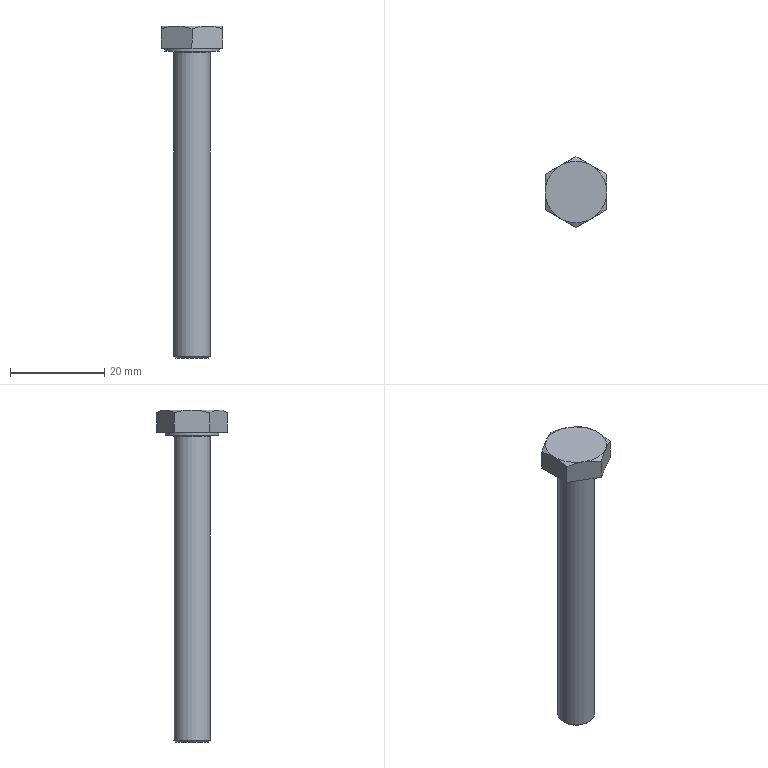Part | NX | features SKETCH 4, EXTRUDE 3, META 3, DATUM_CSYS 2, BLEND 1, CHAMFER 1, LINE 1, SWP104 1, SYMBOLIC_THREAD 1, THREADS 1 | 1 solid | 20 faces | box 13 x 15.011 x 70.3 mm | volume 3821 mm3 | plane 10 | cone 7 | cylinder 2 | torus 1 | commonest cylinder face diameters 7.76 x1 11.47 x1
STEP:
#1=CARTESIAN_POINT('',(4.28,0.,0.));
#2=VERTEX_POINT('',#1);
#3=CARTESIAN_POINT('',(0.,0.,0.));
#4=DIRECTION('',(0.,0.,1.));
#5=DIRECTION('',(1.,0.,0.));
#6=AXIS2_PLACEMENT_3D('',#3,#4,#5);
#7=CIRCLE('',#6,4.28);
#8=EDGE_CURVE('',#2,#2,#7,.T.);
#9=ORIENTED_EDGE('',*,*,#8,.T.);
#10=EDGE_LOOP('',(#9));
#11=FACE_BOUND('',#10,.T.);
#12=CARTESIAN_POINT('',(5.735,0.,0.));
#13=VERTEX_POINT('',#12);
#14=CARTESIAN_POINT('',(0.,0.,0.));
#15=DIRECTION('',(0.,0.,1.));
#16=DIRECTION('',(1.,0.,0.));
#17=AXIS2_PLACEMENT_3D('',#14,#15,#16);
#18=CIRCLE('',#17,5.735);
#19=EDGE_CURVE('',#13,#13,#18,.T.);
#20=ORIENTED_EDGE('',*,*,#19,.F.);
#21=EDGE_LOOP('',(#20));
#22=FACE_BOUND('',#21,.T.);
#23=CARTESIAN_POINT('',(0.,0.,0.));
#24=DIRECTION('',(0.,0.,1.));
#25=DIRECTION('',(1.,0.,0.));
#26=AXIS2_PLACEMENT_3D('',#23,#24,#25);
#27=PLANE('',#26);
#28=ADVANCED_FACE('',(#11,#22),#27,.F.);
#29=CARTESIAN_POINT('',(6.5,3.753,4.719));
#30=VERTEX_POINT('',#29);
#31=CARTESIAN_POINT('',(3.25,5.629,5.3));
#32=VERTEX_POINT('',#31);
#33=CARTESIAN_POINT('',(6.5,3.753,4.719));
#34=CARTESIAN_POINT('',(5.437,4.367,5.074));
#35=CARTESIAN_POINT('',(4.357,4.99,5.3));
#36=CARTESIAN_POINT('',(3.25,5.629,5.3));
#37=B_SPLINE_CURVE_WITH_KNOTS('',3,(#33,#34,#35,#36),.UNSPECIFIED.,.F.,.F.,(4,4),(0.000000238,0.003797),.UNSPECIFIED.);
#38=EDGE_CURVE('',#30,#32,#37,.T.);
#39=ORIENTED_EDGE('',*,*,#38,.F.);
#40=CARTESIAN_POINT('',(6.5,3.753,0.6));
#41=VERTEX_POINT('',#40);
#42=CARTESIAN_POINT('',(6.5,3.753,5.3));
#43=DIRECTION('',(0.,0.,-1.));
#44=VECTOR('',#43,1000.);
#45=LINE('',#42,#44);
#46=EDGE_CURVE('',#30,#41,#45,.T.);
#47=ORIENTED_EDGE('',*,*,#46,.T.);
#48=CARTESIAN_POINT('',(0.,7.506,0.6));
#49=VERTEX_POINT('',#48);
#50=CARTESIAN_POINT('',(0.,7.506,0.6));
#51=DIRECTION('',(0.866,-0.5,0.));
#52=VECTOR('',#51,1000.);
#53=LINE('',#50,#52);
#54=EDGE_CURVE('',#49,#41,#53,.T.);
#55=ORIENTED_EDGE('',*,*,#54,.F.);
#56=CARTESIAN_POINT('',(0.,7.506,4.719));
#57=VERTEX_POINT('',#56);
#58=CARTESIAN_POINT('',(0.,7.506,5.3));
#59=DIRECTION('',(0.,0.,-1.));
#60=VECTOR('',#59,1000.);
#61=LINE('',#58,#60);
#62=EDGE_CURVE('',#57,#49,#61,.T.);
#63=ORIENTED_EDGE('',*,*,#62,.F.);
#64=CARTESIAN_POINT('',(3.25,5.629,5.3));
#65=CARTESIAN_POINT('',(2.147,6.266,5.3));
#66=CARTESIAN_POINT('',(1.061,6.893,5.073));
#67=CARTESIAN_POINT('',(0.,7.506,4.719));
#68=B_SPLINE_CURVE_WITH_KNOTS('',3,(#64,#65,#66,#67),.UNSPECIFIED.,.F.,.F.,(4,4),(0.003797,0.00758),.UNSPECIFIED.);
#69=EDGE_CURVE('',#32,#57,#68,.T.);
#70=ORIENTED_EDGE('',*,*,#69,.F.);
#71=EDGE_LOOP('',(#39,#47,#55,#63,#70));
#72=FACE_BOUND('',#71,.T.);
#73=CARTESIAN_POINT('',(0.,7.506,5.3));
#74=DIRECTION('',(0.5,0.866,0.));
#75=DIRECTION('',(-0.866,0.5,0.));
#76=AXIS2_PLACEMENT_3D('',#73,#74,#75);
#77=PLANE('',#76);
#78=ADVANCED_FACE('',(#72),#77,.T.);
#79=CARTESIAN_POINT('',(6.5,-3.753,4.719));
#80=VERTEX_POINT('',#79);
#81=CARTESIAN_POINT('',(6.5,0.,5.3));
#82=VERTEX_POINT('',#81);
#83=CARTESIAN_POINT('',(6.5,-3.753,4.719));
#84=CARTESIAN_POINT('',(6.5,-2.532,5.072));
#85=CARTESIAN_POINT('',(6.5,-1.268,5.3));
#86=CARTESIAN_POINT('',(6.5,0.,5.3));
#87=B_SPLINE_CURVE_WITH_KNOTS('',3,(#83,#84,#85,#86),.UNSPECIFIED.,.F.,.F.,(4,4),(0.006695,0.01049),.UNSPECIFIED.);
#88=EDGE_CURVE('',#80,#82,#87,.T.);
#89=ORIENTED_EDGE('',*,*,#88,.F.);
#90=CARTESIAN_POINT('',(6.5,-3.753,0.6));
#91=VERTEX_POINT('',#90);
#92=CARTESIAN_POINT('',(6.5,-3.753,5.3));
#93=DIRECTION('',(0.,0.,-1.));
#94=VECTOR('',#93,1000.);
#95=LINE('',#92,#94);
#96=EDGE_CURVE('',#80,#91,#95,.T.);
#97=ORIENTED_EDGE('',*,*,#96,.T.);
#98=CARTESIAN_POINT('',(6.5,3.753,0.6));
#99=DIRECTION('',(0.,-1.,0.));
#100=VECTOR('',#99,1000.);
#101=LINE('',#98,#100);
#102=EDGE_CURVE('',#41,#91,#101,.T.);
#103=ORIENTED_EDGE('',*,*,#102,.F.);
#104=ORIENTED_EDGE('',*,*,#46,.F.);
#105=CARTESIAN_POINT('',(6.5,0.,5.3));
#106=CARTESIAN_POINT('',(6.5,1.269,5.3));
#107=CARTESIAN_POINT('',(6.5,2.539,5.07));
#108=CARTESIAN_POINT('',(6.5,3.753,4.719));
#109=B_SPLINE_CURVE_WITH_KNOTS('',3,(#105,#106,#107,#108),.UNSPECIFIED.,.F.,.F.,(4,4),(0.01049,0.01429),.UNSPECIFIED.);
#110=EDGE_CURVE('',#82,#30,#109,.T.);
#111=ORIENTED_EDGE('',*,*,#110,.F.);
#112=EDGE_LOOP('',(#89,#97,#103,#104,#111));
#113=FACE_BOUND('',#112,.T.);
#114=CARTESIAN_POINT('',(6.5,3.753,5.3));
#115=DIRECTION('',(1.,0.,0.));
#116=DIRECTION('',(0.,0.,-1.));
#117=AXIS2_PLACEMENT_3D('',#114,#115,#116);
#118=PLANE('',#117);
#119=ADVANCED_FACE('',(#113),#118,.T.);
#120=CARTESIAN_POINT('',(0.,-7.506,4.719));
#121=VERTEX_POINT('',#120);
#122=CARTESIAN_POINT('',(3.25,-5.629,5.3));
#123=VERTEX_POINT('',#122);
#124=CARTESIAN_POINT('',(0.,-7.506,4.719));
#125=CARTESIAN_POINT('',(1.063,-6.892,5.074));
#126=CARTESIAN_POINT('',(2.143,-6.269,5.3));
#127=CARTESIAN_POINT('',(3.25,-5.629,5.3));
#128=B_SPLINE_CURVE_WITH_KNOTS('',3,(#124,#125,#126,#127),.UNSPECIFIED.,.F.,.F.,(4,4),(0.000000238,0.003797),.UNSPECIFIED.);
#129=EDGE_CURVE('',#121,#123,#128,.T.);
#130=ORIENTED_EDGE('',*,*,#129,.F.);
#131=CARTESIAN_POINT('',(0.,-7.506,0.6));
#132=VERTEX_POINT('',#131);
#133=CARTESIAN_POINT('',(0.,-7.506,5.3));
#134=DIRECTION('',(0.,0.,-1.));
#135=VECTOR('',#134,1000.);
#136=LINE('',#133,#135);
#137=EDGE_CURVE('',#121,#132,#136,.T.);
#138=ORIENTED_EDGE('',*,*,#137,.T.);
#139=CARTESIAN_POINT('',(6.5,-3.753,0.6));
#140=DIRECTION('',(-0.866,-0.5,0.));
#141=VECTOR('',#140,1000.);
#142=LINE('',#139,#141);
#143=EDGE_CURVE('',#91,#132,#142,.T.);
#144=ORIENTED_EDGE('',*,*,#143,.F.);
#145=ORIENTED_EDGE('',*,*,#96,.F.);
#146=CARTESIAN_POINT('',(3.25,-5.629,5.3));
#147=CARTESIAN_POINT('',(4.353,-4.992,5.3));
#148=CARTESIAN_POINT('',(5.439,-4.365,5.073));
#149=CARTESIAN_POINT('',(6.5,-3.753,4.719));
#150=B_SPLINE_CURVE_WITH_KNOTS('',3,(#146,#147,#148,#149),.UNSPECIFIED.,.F.,.F.,(4,4),(0.003797,0.00758),.UNSPECIFIED.);
#151=EDGE_CURVE('',#123,#80,#150,.T.);
#152=ORIENTED_EDGE('',*,*,#151,.F.);
#153=EDGE_LOOP('',(#130,#138,#144,#145,#152));
#154=FACE_BOUND('',#153,.T.);
#155=CARTESIAN_POINT('',(6.5,-3.753,5.3));
#156=DIRECTION('',(0.5,-0.866,0.));
#157=DIRECTION('',(0.866,0.5,0.));
#158=AXIS2_PLACEMENT_3D('',#155,#156,#157);
#159=PLANE('',#158);
#160=ADVANCED_FACE('',(#154),#159,.T.);
#161=CARTESIAN_POINT('',(-6.5,-3.753,4.719));
#162=VERTEX_POINT('',#161);
#163=CARTESIAN_POINT('',(-3.25,-5.629,5.3));
#164=VERTEX_POINT('',#163);
#165=CARTESIAN_POINT('',(-6.5,-3.753,4.719));
#166=CARTESIAN_POINT('',(-5.437,-4.367,5.074));
#167=CARTESIAN_POINT('',(-4.357,-4.99,5.3));
#168=CARTESIAN_POINT('',(-3.25,-5.629,5.3));
#169=B_SPLINE_CURVE_WITH_KNOTS('',3,(#165,#166,#167,#168),.UNSPECIFIED.,.F.,.F.,(4,4),(0.000000238,0.003797),.UNSPECIFIED.);
#170=EDGE_CURVE('',#162,#164,#169,.T.);
#171=ORIENTED_EDGE('',*,*,#170,.F.);
#172=CARTESIAN_POINT('',(-6.5,-3.753,0.6));
#173=VERTEX_POINT('',#172);
#174=CARTESIAN_POINT('',(-6.5,-3.753,5.3));
#175=DIRECTION('',(0.,0.,-1.));
#176=VECTOR('',#175,1000.);
#177=LINE('',#174,#176);
#178=EDGE_CURVE('',#162,#173,#177,.T.);
#179=ORIENTED_EDGE('',*,*,#178,.T.);
#180=CARTESIAN_POINT('',(0.,-7.506,0.6));
#181=DIRECTION('',(-0.866,0.5,0.));
#182=VECTOR('',#181,1000.);
#183=LINE('',#180,#182);
#184=EDGE_CURVE('',#132,#173,#183,.T.);
#185=ORIENTED_EDGE('',*,*,#184,.F.);
#186=ORIENTED_EDGE('',*,*,#137,.F.);
#187=CARTESIAN_POINT('',(-3.25,-5.629,5.3));
#188=CARTESIAN_POINT('',(-2.147,-6.266,5.3));
#189=CARTESIAN_POINT('',(-1.061,-6.893,5.073));
#190=CARTESIAN_POINT('',(0.,-7.506,4.719));
#191=B_SPLINE_CURVE_WITH_KNOTS('',3,(#187,#188,#189,#190),.UNSPECIFIED.,.F.,.F.,(4,4),(0.003797,0.00758),.UNSPECIFIED.);
#192=EDGE_CURVE('',#164,#121,#191,.T.);
#193=ORIENTED_EDGE('',*,*,#192,.F.);
#194=EDGE_LOOP('',(#171,#179,#185,#186,#193));
#195=FACE_BOUND('',#194,.T.);
#196=CARTESIAN_POINT('',(0.,-7.506,5.3));
#197=DIRECTION('',(-0.5,-0.866,0.));
#198=DIRECTION('',(0.866,-0.5,0.));
#199=AXIS2_PLACEMENT_3D('',#196,#197,#198);
#200=PLANE('',#199);
#201=ADVANCED_FACE('',(#195),#200,.T.);
#202=CARTESIAN_POINT('',(-6.5,3.753,4.719));
#203=VERTEX_POINT('',#202);
#204=CARTESIAN_POINT('',(-6.5,0.,5.3));
#205=VERTEX_POINT('',#204);
#206=CARTESIAN_POINT('',(-6.5,0.,5.3));
#207=CARTESIAN_POINT('',(-6.5,1.269,5.3));
#208=CARTESIAN_POINT('',(-6.5,2.539,5.07));
#209=CARTESIAN_POINT('',(-6.5,3.753,4.719));
#210=B_SPLINE_CURVE_WITH_KNOTS('',3,(#206,#207,#208,#209),.UNSPECIFIED.,.F.,.F.,(4,4),(0.01049,0.01429),.UNSPECIFIED.);
#211=EDGE_CURVE('',#203,#205,#210,.F.);
#212=ORIENTED_EDGE('',*,*,#211,.F.);
#213=CARTESIAN_POINT('',(-6.5,3.753,0.6));
#214=VERTEX_POINT('',#213);
#215=CARTESIAN_POINT('',(-6.5,3.753,5.3));
#216=DIRECTION('',(0.,0.,-1.));
#217=VECTOR('',#216,1000.);
#218=LINE('',#215,#217);
#219=EDGE_CURVE('',#203,#214,#218,.T.);
#220=ORIENTED_EDGE('',*,*,#219,.T.);
#221=CARTESIAN_POINT('',(-6.5,-3.753,0.6));
#222=DIRECTION('',(0.,1.,0.));
#223=VECTOR('',#222,1000.);
#224=LINE('',#221,#223);
#225=EDGE_CURVE('',#173,#214,#224,.T.);
#226=ORIENTED_EDGE('',*,*,#225,.F.);
#227=ORIENTED_EDGE('',*,*,#178,.F.);
#228=CARTESIAN_POINT('',(-6.5,-3.753,4.719));
#229=CARTESIAN_POINT('',(-6.5,-2.532,5.072));
#230=CARTESIAN_POINT('',(-6.5,-1.268,5.3));
#231=CARTESIAN_POINT('',(-6.5,0.,5.3));
#232=B_SPLINE_CURVE_WITH_KNOTS('',3,(#228,#229,#230,#231),.UNSPECIFIED.,.F.,.F.,(4,4),(0.006695,0.01049),.UNSPECIFIED.);
#233=EDGE_CURVE('',#205,#162,#232,.F.);
#234=ORIENTED_EDGE('',*,*,#233,.F.);
#235=EDGE_LOOP('',(#212,#220,#226,#227,#234));
#236=FACE_BOUND('',#235,.T.);
#237=CARTESIAN_POINT('',(-6.5,-3.753,5.3));
#238=DIRECTION('',(-1.,0.,0.));
#239=DIRECTION('',(0.,0.,1.));
#240=AXIS2_PLACEMENT_3D('',#237,#238,#239);
#241=PLANE('',#240);
#242=ADVANCED_FACE('',(#236),#241,.T.);
#243=CARTESIAN_POINT('',(-3.25,5.629,5.3));
#244=VERTEX_POINT('',#243);
#245=CARTESIAN_POINT('',(0.,7.506,4.719));
#246=CARTESIAN_POINT('',(-1.063,6.892,5.074));
#247=CARTESIAN_POINT('',(-2.143,6.269,5.3));
#248=CARTESIAN_POINT('',(-3.25,5.629,5.3));
#249=B_SPLINE_CURVE_WITH_KNOTS('',3,(#245,#246,#247,#248),.UNSPECIFIED.,.F.,.F.,(4,4),(0.000000238,0.003797),.UNSPECIFIED.);
#250=EDGE_CURVE('',#57,#244,#249,.T.);
#251=ORIENTED_EDGE('',*,*,#250,.F.);
#252=ORIENTED_EDGE('',*,*,#62,.T.);
#253=CARTESIAN_POINT('',(-6.5,3.753,0.6));
#254=DIRECTION('',(0.866,0.5,0.));
#255=VECTOR('',#254,1000.);
#256=LINE('',#253,#255);
#257=EDGE_CURVE('',#214,#49,#256,.T.);
#258=ORIENTED_EDGE('',*,*,#257,.F.);
#259=ORIENTED_EDGE('',*,*,#219,.F.);
#260=CARTESIAN_POINT('',(-3.25,5.629,5.3));
#261=CARTESIAN_POINT('',(-4.353,4.992,5.3));
#262=CARTESIAN_POINT('',(-5.439,4.365,5.073));
#263=CARTESIAN_POINT('',(-6.5,3.753,4.719));
#264=B_SPLINE_CURVE_WITH_KNOTS('',3,(#260,#261,#262,#263),.UNSPECIFIED.,.F.,.F.,(4,4),(0.003797,0.00758),.UNSPECIFIED.);
#265=EDGE_CURVE('',#244,#203,#264,.T.);
#266=ORIENTED_EDGE('',*,*,#265,.F.);
#267=EDGE_LOOP('',(#251,#252,#258,#259,#266));
#268=FACE_BOUND('',#267,.T.);
#269=CARTESIAN_POINT('',(-6.5,3.753,5.3));
#270=DIRECTION('',(-0.5,0.866,0.));
#271=DIRECTION('',(-0.866,-0.5,0.));
#272=AXIS2_PLACEMENT_3D('',#269,#270,#271);
#273=PLANE('',#272);
#274=ADVANCED_FACE('',(#268),#273,.T.);
#275=CARTESIAN_POINT('',(5.735,0.,0.6));
#276=VERTEX_POINT('',#275);
#277=CARTESIAN_POINT('',(0.,0.,0.6));
#278=DIRECTION('',(0.,0.,1.));
#279=DIRECTION('',(1.,0.,0.));
#280=AXIS2_PLACEMENT_3D('',#277,#278,#279);
#281=CIRCLE('',#280,5.735);
#282=EDGE_CURVE('',#276,#276,#281,.T.);
#283=ORIENTED_EDGE('',*,*,#282,.T.);
#284=EDGE_LOOP('',(#283));
#285=FACE_BOUND('',#284,.T.);
#286=ORIENTED_EDGE('',*,*,#54,.T.);
#287=ORIENTED_EDGE('',*,*,#102,.T.);
#288=ORIENTED_EDGE('',*,*,#143,.T.);
#289=ORIENTED_EDGE('',*,*,#184,.T.);
#290=ORIENTED_EDGE('',*,*,#225,.T.);
#291=ORIENTED_EDGE('',*,*,#257,.T.);
#292=EDGE_LOOP('',(#286,#287,#288,#289,#290,#291));
#293=FACE_BOUND('',#292,.T.);
#294=CARTESIAN_POINT('',(0.,7.506,0.6));
#295=DIRECTION('',(0.,0.,1.));
#296=DIRECTION('',(1.,0.,0.));
#297=AXIS2_PLACEMENT_3D('',#294,#295,#296);
#298=PLANE('',#297);
#299=ADVANCED_FACE('',(#285,#293),#298,.F.);
#300=ORIENTED_EDGE('',*,*,#282,.F.);
#301=EDGE_LOOP('',(#300));
#302=FACE_BOUND('',#301,.T.);
#303=ORIENTED_EDGE('',*,*,#19,.T.);
#304=EDGE_LOOP('',(#303));
#305=FACE_BOUND('',#304,.T.);
#306=CARTESIAN_POINT('',(0.,0.,0.6));
#307=DIRECTION('',(0.,0.,-1.));
#308=DIRECTION('',(-1.,0.,0.));
#309=AXIS2_PLACEMENT_3D('',#306,#307,#308);
#310=CYLINDRICAL_SURFACE('',#309,5.735);
#311=ADVANCED_FACE('',(#302,#305),#310,.T.);
#312=CARTESIAN_POINT('',(-3.88,0.,-64.612));
#313=VERTEX_POINT('',#312);
#314=CARTESIAN_POINT('',(0.,0.,-64.612));
#315=DIRECTION('',(0.,0.,-1.));
#316=DIRECTION('',(-1.,0.,0.));
#317=AXIS2_PLACEMENT_3D('',#314,#315,#316);
#318=CIRCLE('',#317,3.88);
#319=EDGE_CURVE('',#313,#313,#318,.F.);
#320=ORIENTED_EDGE('',*,*,#319,.T.);
#321=EDGE_LOOP('',(#320));
#322=FACE_BOUND('',#321,.T.);
#323=CARTESIAN_POINT('',(3.88,0.,-0.4));
#324=VERTEX_POINT('',#323);
#325=CARTESIAN_POINT('',(0.,0.,-0.4));
#326=DIRECTION('',(0.,0.,1.));
#327=DIRECTION('',(1.,0.,0.));
#328=AXIS2_PLACEMENT_3D('',#325,#326,#327);
#329=CIRCLE('',#328,3.88);
#330=EDGE_CURVE('',#324,#324,#329,.F.);
#331=ORIENTED_EDGE('',*,*,#330,.T.);
#332=EDGE_LOOP('',(#331));
#333=FACE_BOUND('',#332,.T.);
#334=CARTESIAN_POINT('',(0.,0.,-65.));
#335=DIRECTION('',(0.,0.,1.));
#336=DIRECTION('',(1.,0.,0.));
#337=AXIS2_PLACEMENT_3D('',#334,#335,#336);
#338=CYLINDRICAL_SURFACE('',#337,3.88);
#339=ADVANCED_FACE('',(#322,#333),#338,.T.);
#340=CARTESIAN_POINT('',(-3.492,0.,-65.));
#341=VERTEX_POINT('',#340);
#342=CARTESIAN_POINT('',(0.,0.,-65.));
#343=DIRECTION('',(0.,0.,-1.));
#344=DIRECTION('',(-1.,0.,0.));
#345=AXIS2_PLACEMENT_3D('',#342,#343,#344);
#346=CIRCLE('',#345,3.492);
#347=EDGE_CURVE('',#341,#341,#346,.T.);
#348=ORIENTED_EDGE('',*,*,#347,.T.);
#349=EDGE_LOOP('',(#348));
#350=FACE_BOUND('',#349,.T.);
#351=CARTESIAN_POINT('',(0.,0.,-65.));
#352=DIRECTION('',(0.,0.,-1.));
#353=DIRECTION('',(-1.,0.,0.));
#354=AXIS2_PLACEMENT_3D('',#351,#352,#353);
#355=PLANE('',#354);
#356=ADVANCED_FACE('',(#350),#355,.T.);
#357=ORIENTED_EDGE('',*,*,#211,.T.);
#358=CARTESIAN_POINT('',(0.,0.,5.3));
#359=DIRECTION('',(0.,0.,-1.));
#360=DIRECTION('',(-1.,0.,0.));
#361=AXIS2_PLACEMENT_3D('',#358,#359,#360);
#362=CIRCLE('',#361,6.5);
#363=EDGE_CURVE('',#205,#244,#362,.T.);
#364=ORIENTED_EDGE('',*,*,#363,.T.);
#365=ORIENTED_EDGE('',*,*,#265,.T.);
#366=EDGE_LOOP('',(#357,#364,#365));
#367=FACE_BOUND('',#366,.T.);
#368=CARTESIAN_POINT('',(0.,0.,5.3));
#369=DIRECTION('',(0.,0.,-1.));
#370=DIRECTION('',(-1.,0.,0.));
#371=AXIS2_PLACEMENT_3D('',#368,#369,#370);
#372=CONICAL_SURFACE('',#371,6.5,1.047);
#373=ADVANCED_FACE('',(#367),#372,.T.);
#374=ORIENTED_EDGE('',*,*,#69,.T.);
#375=ORIENTED_EDGE('',*,*,#250,.T.);
#376=CARTESIAN_POINT('',(0.,0.,5.3));
#377=DIRECTION('',(0.,0.,-1.));
#378=DIRECTION('',(-1.,0.,0.));
#379=AXIS2_PLACEMENT_3D('',#376,#377,#378);
#380=CIRCLE('',#379,6.5);
#381=EDGE_CURVE('',#244,#32,#380,.T.);
#382=ORIENTED_EDGE('',*,*,#381,.T.);
#383=EDGE_LOOP('',(#374,#375,#382));
#384=FACE_BOUND('',#383,.T.);
#385=CARTESIAN_POINT('',(0.,0.,5.3));
#386=DIRECTION('',(0.,0.,-1.));
#387=DIRECTION('',(-1.,0.,0.));
#388=AXIS2_PLACEMENT_3D('',#385,#386,#387);
#389=CONICAL_SURFACE('',#388,6.5,1.047);
#390=ADVANCED_FACE('',(#384),#389,.T.);
#391=ORIENTED_EDGE('',*,*,#170,.T.);
#392=CARTESIAN_POINT('',(0.,0.,5.3));
#393=DIRECTION('',(0.,0.,-1.));
#394=DIRECTION('',(-1.,0.,0.));
#395=AXIS2_PLACEMENT_3D('',#392,#393,#394);
#396=CIRCLE('',#395,6.5);
#397=EDGE_CURVE('',#164,#205,#396,.T.);
#398=ORIENTED_EDGE('',*,*,#397,.T.);
#399=ORIENTED_EDGE('',*,*,#233,.T.);
#400=EDGE_LOOP('',(#391,#398,#399));
#401=FACE_BOUND('',#400,.T.);
#402=CARTESIAN_POINT('',(0.,0.,5.3));
#403=DIRECTION('',(0.,0.,-1.));
#404=DIRECTION('',(-1.,0.,0.));
#405=AXIS2_PLACEMENT_3D('',#402,#403,#404);
#406=CONICAL_SURFACE('',#405,6.5,1.047);
#407=ADVANCED_FACE('',(#401),#406,.T.);
#408=ORIENTED_EDGE('',*,*,#129,.T.);
#409=CARTESIAN_POINT('',(0.,0.,5.3));
#410=DIRECTION('',(0.,0.,-1.));
#411=DIRECTION('',(-1.,0.,0.));
#412=AXIS2_PLACEMENT_3D('',#409,#410,#411);
#413=CIRCLE('',#412,6.5);
#414=EDGE_CURVE('',#123,#164,#413,.T.);
#415=ORIENTED_EDGE('',*,*,#414,.T.);
#416=ORIENTED_EDGE('',*,*,#192,.T.);
#417=EDGE_LOOP('',(#408,#415,#416));
#418=FACE_BOUND('',#417,.T.);
#419=CARTESIAN_POINT('',(0.,0.,5.3));
#420=DIRECTION('',(0.,0.,-1.));
#421=DIRECTION('',(-1.,0.,0.));
#422=AXIS2_PLACEMENT_3D('',#419,#420,#421);
#423=CONICAL_SURFACE('',#422,6.5,1.047);
#424=ADVANCED_FACE('',(#418),#423,.T.);
#425=ORIENTED_EDGE('',*,*,#151,.T.);
#426=ORIENTED_EDGE('',*,*,#88,.T.);
#427=CARTESIAN_POINT('',(0.,0.,5.3));
#428=DIRECTION('',(0.,0.,-1.));
#429=DIRECTION('',(-1.,0.,0.));
#430=AXIS2_PLACEMENT_3D('',#427,#428,#429);
#431=CIRCLE('',#430,6.5);
#432=EDGE_CURVE('',#82,#123,#431,.T.);
#433=ORIENTED_EDGE('',*,*,#432,.T.);
#434=EDGE_LOOP('',(#425,#426,#433));
#435=FACE_BOUND('',#434,.T.);
#436=CARTESIAN_POINT('',(0.,0.,5.3));
#437=DIRECTION('',(0.,0.,-1.));
#438=DIRECTION('',(-1.,0.,0.));
#439=AXIS2_PLACEMENT_3D('',#436,#437,#438);
#440=CONICAL_SURFACE('',#439,6.5,1.047);
#441=ADVANCED_FACE('',(#435),#440,.T.);
#442=ORIENTED_EDGE('',*,*,#110,.T.);
#443=ORIENTED_EDGE('',*,*,#38,.T.);
#444=CARTESIAN_POINT('',(0.,0.,5.3));
#445=DIRECTION('',(0.,0.,-1.));
#446=DIRECTION('',(-1.,0.,0.));
#447=AXIS2_PLACEMENT_3D('',#444,#445,#446);
#448=CIRCLE('',#447,6.5);
#449=EDGE_CURVE('',#32,#82,#448,.T.);
#450=ORIENTED_EDGE('',*,*,#449,.T.);
#451=EDGE_LOOP('',(#442,#443,#450));
#452=FACE_BOUND('',#451,.T.);
#453=CARTESIAN_POINT('',(0.,0.,5.3));
#454=DIRECTION('',(0.,0.,-1.));
#455=DIRECTION('',(-1.,0.,0.));
#456=AXIS2_PLACEMENT_3D('',#453,#454,#455);
#457=CONICAL_SURFACE('',#456,6.5,1.047);
#458=ADVANCED_FACE('',(#452),#457,.T.);
#459=ORIENTED_EDGE('',*,*,#363,.F.);
#460=ORIENTED_EDGE('',*,*,#397,.F.);
#461=ORIENTED_EDGE('',*,*,#414,.F.);
#462=ORIENTED_EDGE('',*,*,#432,.F.);
#463=ORIENTED_EDGE('',*,*,#449,.F.);
#464=ORIENTED_EDGE('',*,*,#381,.F.);
#465=EDGE_LOOP('',(#459,#460,#461,#462,#463,#464));
#466=FACE_BOUND('',#465,.T.);
#467=CARTESIAN_POINT('',(0.,7.506,5.3));
#468=DIRECTION('',(0.,0.,1.));
#469=DIRECTION('',(1.,0.,0.));
#470=AXIS2_PLACEMENT_3D('',#467,#468,#469);
#471=PLANE('',#470);
#472=ADVANCED_FACE('',(#466),#471,.T.);
#473=ORIENTED_EDGE('',*,*,#8,.F.);
#474=EDGE_LOOP('',(#473));
#475=FACE_BOUND('',#474,.T.);
#476=ORIENTED_EDGE('',*,*,#330,.F.);
#477=EDGE_LOOP('',(#476));
#478=FACE_BOUND('',#477,.T.);
#479=CARTESIAN_POINT('',(0.,0.,-0.4));
#480=DIRECTION('',(0.,0.,1.));
#481=DIRECTION('',(1.,0.,0.));
#482=AXIS2_PLACEMENT_3D('',#479,#480,#481);
#483=TOROIDAL_SURFACE('',#482,4.28,0.4);
#484=ADVANCED_FACE('',(#475,#478),#483,.F.);
#485=ORIENTED_EDGE('',*,*,#319,.F.);
#486=EDGE_LOOP('',(#485));
#487=FACE_BOUND('',#486,.T.);
#488=ORIENTED_EDGE('',*,*,#347,.F.);
#489=EDGE_LOOP('',(#488));
#490=FACE_BOUND('',#489,.T.);
#491=CARTESIAN_POINT('',(0.,0.,-65.));
#492=DIRECTION('',(0.,0.,1.));
#493=DIRECTION('',(1.,0.,0.));
#494=AXIS2_PLACEMENT_3D('',#491,#492,#493);
#495=CONICAL_SURFACE('',#494,3.492,0.7854);
#496=ADVANCED_FACE('',(#487,#490),#495,.T.);
#497=CLOSED_SHELL('',(#28,#78,#119,#160,#201,#242,#274,#299,#311,#339,#356,#373,#390,#407,#424,#441,#458,#472,#484,#496));
#498=MANIFOLD_SOLID_BREP('',#497);
#499=(LENGTH_UNIT()NAMED_UNIT(*)SI_UNIT(.MILLI.,.METRE.));
#500=UNCERTAINTY_MEASURE_WITH_UNIT(LENGTH_MEASURE(0.0508),#499,'','');
#501=(NAMED_UNIT(*)PLANE_ANGLE_UNIT()SI_UNIT($,.RADIAN.));
#502=(NAMED_UNIT(*)SI_UNIT($,.STERADIAN.)SOLID_ANGLE_UNIT());
#503=(GEOMETRIC_REPRESENTATION_CONTEXT(3)GLOBAL_UNCERTAINTY_ASSIGNED_CONTEXT((#500))GLOBAL_UNIT_ASSIGNED_CONTEXT((#499,#501,#502))REPRESENTATION_CONTEXT('',''));
#504=ADVANCED_BREP_SHAPE_REPRESENTATION('',(#498),#503);